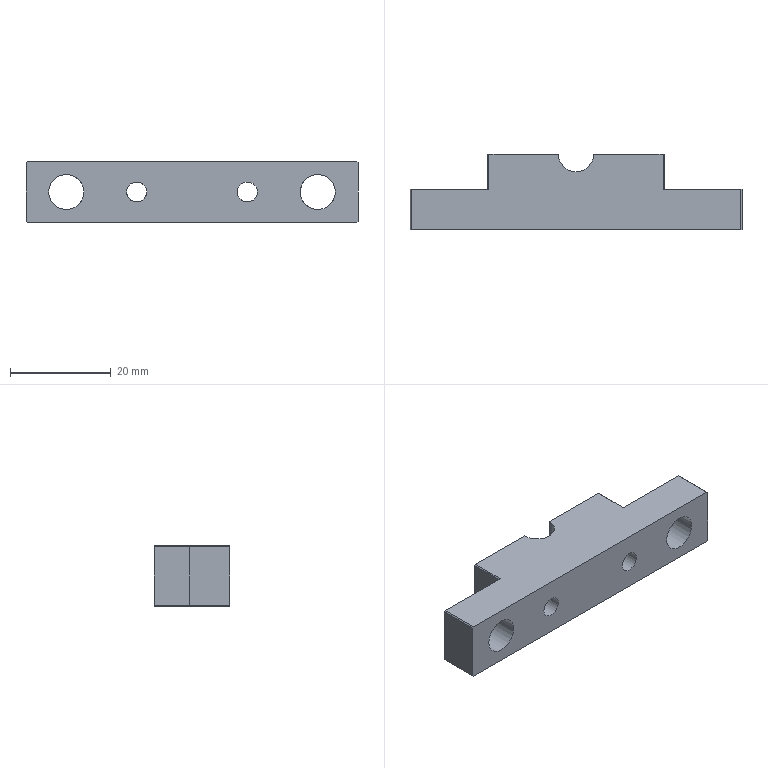NC program | NX | posted with a generic post | part box 66 x 15 x 12 mm
Whole program:
N10 G17 G21 G94 G90
(PLANAR_MILL , TOOL : D10开粗)
N12 T02 M6
N14 G54
N16 G17 G0 G90 X46.5 Y-3. B0. C0. S4500 M3
N18 G43 Z30. H2
N20 Z2.
N22 G94 G1 Z0. F1000.
N24 X36.5
N26 X-36.5
N28 X-46.5
N30 Z2.
N32 G0 Z30.
N34 X46.5 Y3.
N36 Z2.
N38 G1 Z0.
N40 X36.5
N42 X-36.5
N44 X-46.5
N46 Z2.
N48 G0 Z30.
(ADAPTIVE_MILLING , TOOL : D10开粗)
N50 X-32.154 Y-18.537 S5500
N52 Z-13.
N54 G1 X-32.171 Y-18.388 Z-13.937 F3000.
N56 X-32.188 Y-18.239 Z-14.308
N58 X-32.205 Y-18.09 Z-14.58
N60 X-32.222 Y-17.941 Z-14.8
N62 X-32.239 Y-17.791 Z-14.984
N64 X-32.255 Y-17.642 Z-15.142
N66 X-32.272 Y-17.493 Z-15.28
N68 X-32.289 Y-17.344 Z-15.4
N70 X-32.306 Y-17.195 Z-15.505
N72 X-32.323 Y-17.046 Z-15.598
N74 X-32.339 Y-16.897 Z-15.679
N76 X-32.356 Y-16.748 Z-15.75
N78 X-32.373 Y-16.599 Z-15.81
N80 X-32.39 Y-16.45 Z-15.862
N82 X-32.407 Y-16.301 Z-15.905
N84 X-32.424 Y-16.152 Z-15.939
N86 X-32.44 Y-16.003 Z-15.966
N88 X-32.457 Y-15.854 Z-15.985
N90 X-32.474 Y-15.705 Z-15.996
N92 X-32.491 Y-15.556 Z-16.
N94 X-32.687 Y-13.82
N96 G3 X-33.155 Y-13.077 R1.012
N98 X-34.636 Y-12.384 R5.494
N100 G2 X-37.759 Y-9.525 R6.545
N102 X-39.326 Y-4.936 R13.806
N104 X-39.908 Y3.097 R49.25
N106 X-39.899 Y5.158 R31.931
N108 X-37.912 Y8.459 R5.464
N110 G3 X-37.184 Y9.047 R22.941
N112 G2 X-34.827 Y10.897 R6.19
N114 X-32.799 Y11.3 R6.2
N116 X-22.302 Y11.491 R214.981
N118 G1 X-12.927 Y11.5
N120 X33.391 Y11.49
N122 G2 X36.639 Y9.788 R5.115
N124 X38.854 Y5.697 R9.985
N126 X39.767 Y-0.221 R27.104
N128 X39.889 Y-4.904 R50.965
N130 X38.038 Y-8.275 R5.243
N132 G1 X37.273 Y-8.915
N134 G2 X36.547 Y-9.748 R5.739
N136 X34.827 Y-10.897 R6.197
N138 X32.8 Y-11.3 R6.2
N140 X21.928 Y-11.492 R225.85
N142 G1 X12.928 Y-11.5
N144 X-29.01 Y-11.493
N146 G2 X-30.739 Y-11.3 R10.213
N148 X-33.493 Y-11.252 R28.791
N150 X-34.758 Y-10.925 R9.784
N152 G1 X-35.713 Y-10.428
N154 G2 X-37.407 Y-8.743 R7.579
N156 X-38.198 Y-6.833 R6.195
N158 G1 X-38.3 Y-5.799
N160 Y5.801
N162 G2 X-36.547 Y9.748 R5.488
N164 X-34.827 Y10.897 R6.197
N166 X-32.799 Y11.3 R6.2
N168 G1 X33.031 Y11.293
N170 X33.722 Y11.219
N172 X34.758 Y10.925
N174 X35.713 Y10.428
N176 G2 X37.335 Y8.849 R7.764
N178 X38.3 Y5.8 R5.571
N180 G1 Y-5.801
N182 G2 X36.547 Y-9.748 R5.489
N184 X34.827 Y-10.897 R6.197
N186 X32.8 Y-11.3 R6.2
N188 G1 X-30.763
N190 G3 X-31.772 Y-12.294 R1.01
N192 G1 X-31.796 Y-13.727
N194 X-31.798 Y-13.877 Z-15.996
N196 X-31.8 Y-14.027 Z-15.985
N198 X-31.803 Y-14.177 Z-15.966
N200 X-31.805 Y-14.326 Z-15.939
N202 X-31.808 Y-14.476 Z-15.905
N204 X-31.81 Y-14.626 Z-15.862
N206 X-31.813 Y-14.776 Z-15.81
N208 X-31.815 Y-14.926 Z-15.75
N210 X-31.818 Y-15.076 Z-15.679
N212 X-31.82 Y-15.226 Z-15.598
N214 X-31.822 Y-15.376 Z-15.505
N216 X-31.825 Y-15.526 Z-15.4
N218 X-31.827 Y-15.676 Z-15.28
N220 X-31.83 Y-15.826 Z-15.142
N222 X-31.832 Y-15.976 Z-14.984
N224 X-31.835 Y-16.126 Z-14.8
N226 X-31.837 Y-16.276 Z-14.58
N228 X-31.839 Y-16.426 Z-14.308
N230 X-31.842 Y-16.576 Z-13.937
N232 X-31.844 Y-16.726 Z-13.
N234 G0 Z30.
(PLANAR_MILL_1 , TOOL : D10开粗)
N236 X39.079 Y-11. S4500
N238 Z-14.
N240 G1 Z-16. F800.
N242 X32.799
N244 X-32.8
N246 G2 X-36.336 Y-9.536 R5.
N248 G1 X-36.536 Y-9.336
N250 G2 X-38. Y-5.8 R5.
N252 G1 Y5.8
N254 G2 X-36.536 Y9.336 R5.
N256 G1 X-36.336 Y9.536
N258 G2 X-32.8 Y11. R5.
N260 G1 X32.8
N262 G2 X36.336 Y9.536 R5.
N264 G1 X36.536 Y9.336
N266 G2 X38. Y5.8 R5.
N268 G1 Y-5.8
N270 G2 X36.536 Y-9.336 R5.
N272 G1 X36.336 Y-9.535
N274 X31.871 Y-14.
N276 Z-14.
N278 G0 Z30.
N280 X39.079 Y-11.
N282 Z-14.
N284 G1 Z-16.
N286 X32.799
N288 X-32.8
N290 G2 X-36.336 Y-9.536 R5.
N292 G1 X-36.536 Y-9.336
N294 G2 X-38. Y-5.8 R5.
N296 G1 Y5.8
N298 G2 X-36.536 Y9.336 R5.
N300 G1 X-36.336 Y9.536
N302 G2 X-32.8 Y11. R5.
N304 G1 X32.8
N306 G2 X36.336 Y9.536 R5.
N308 G1 X36.536 Y9.336
N310 G2 X38. Y5.8 R5.
N312 G1 Y-5.8
N314 G2 X36.536 Y-9.336 R5.
N316 G1 X36.336 Y-9.535
N318 X31.871 Y-14.
N320 Z-14.
N322 G0 Z30.
N324 X39.079 Y-11.
N326 Z-14.
N328 G1 Z-16.
N330 X32.799
N332 X-32.8
N334 G2 X-36.336 Y-9.536 R5.
N336 G1 X-36.536 Y-9.336
N338 G2 X-38. Y-5.8 R5.
N340 G1 Y5.8
N342 G2 X-36.536 Y9.336 R5.
N344 G1 X-36.336 Y9.536
N346 G2 X-32.8 Y11. R5.
N348 G1 X32.8
N350 G2 X36.336 Y9.536 R5.
N352 G1 X36.536 Y9.336
N354 G2 X38. Y5.8 R5.
N356 G1 Y-5.8
N358 G2 X36.536 Y-9.336 R5.
N360 G1 X36.336 Y-9.535
N362 X31.871 Y-14.
N364 Z-14.
N366 G0 Z30.
N368 M5
(PLANAR_MILL_1_COPY , TOOL : D8倒角刀)
N370 T04 M6
N372 G54
N374 G17 G0 G90 X36.341 Y-8. B0. C0. S4500 M3
N376 G43 Z30. H4
N378 Z0.
N380 G94 G1 Z-2. F800.
N382 X32.8
N384 X-32.8
N386 G2 X-34.214 Y-7.414 R2.
N388 G1 X-34.414 Y-7.214
N390 G2 X-35. Y-5.8 R2.
N392 G1 Y5.8
N394 G2 X-34.414 Y7.214 R2.
N396 G1 X-34.214 Y7.414
N398 G2 X-32.8 Y8. R2.
N400 G1 X32.8
N402 G2 X34.214 Y7.414 R2.
N404 G1 X34.414 Y7.214
N406 G2 X35. Y5.8 R2.
N408 G1 Y-5.8
N410 G2 X34.414 Y-7.214 R2.
N412 G1 X34.215 Y-7.414
N414 X31.628 Y-10.
N416 Z0.
N418 G0 Z30.
(DRILLING , TOOL : D8倒角刀)
N420 X-25. Y0. S3000
N422 G81 G98 Z-3.5 F200. R3.
N424 X25.
N426 G80
N428 G0 X25. Y0. Z30.
(DRILLING_COPY , TOOL : D8倒角刀)
N430 X-11.
N432 G81 Z-2.1 F200. R3.
N434 X11.
N436 G80
N438 G0 X11. Y0. Z30.
N440 M5
(PLANAR_MILL_COPY , TOOL : D63R0.8)
N442 T01 M6
N444 G54
N446 G17 G0 G90 X73. Y-3.5 B0. C0. S3500 M3
N448 G43 Z30. H1
N450 Z2.
N452 G94 G1 Z0. F600.
N454 X36.5
N456 X-36.5
N458 X-73.
N460 Z2.
N462 G0 Z30.
N464 M5
(DRILLING_COPY_1 , TOOL : D7钻头)
N466 T05 M6
N468 G54
N470 G17 G0 G90 X-25. Y0. B0. C0. S3000 M3
N472 G43 Z30. H5
N474 G94 G83 G98 Z-15. F200. Q2. R3.
N476 X25.
N478 G80
N480 G0 X25. Y0. Z30.
N482 M5
(HOLE_MILLING , TOOL : D4开粗)
N484 T08 M6
N486 G54
N488 G17 G0 G90 X-25. Y0. B0. C0. S4500 M3
N490 G43 Z30. H8
N492 Z-9.
N494 G94 G3 X-24.25 Y-0.75 R0.75 F200.
N496 X-23.5 Y0. R0.75
N498 X-25. Y1.5 R1.5
N500 X-23.5 Y0. R-1.5
N502 X-24.25 Y0.75 R0.75
N504 X-25. Y0. R0.75
N506 G0 Z30.
N508 X25.
N510 Z-9.
N512 G3 X25.75 Y-0.75 R0.75
N514 X26.5 Y0. R0.75
N516 X25. Y1.5 R1.5
N518 X26.5 Y0. R-1.5
N520 X25.75 Y0.75 R0.75
N522 X25. Y0. R0.75
N524 G0 Z30.
N526 M5
(DRILLING_COPY_COPY , TOOL : Z3.3)
N528 T06 M6
N530 G54
N532 G17 G0 G90 X-11. Y0. B0. C0. S3000 M3
N534 G43 Z30. H6
N536 G94 G83 G98 Z-18. F200. Q2. R3.
N538 X11.
N540 G80
N542 G0 X11. Y0. Z30.
N544 M5
(DRILLING_COPY_COPY_COPY , TOOL : M4X0.7)
N546 T07 M6
N548 G54
N550 G17 G0 G90 X-11. Y0. B0. C0. S300 M3
N552 G43 Z30. H7
N554 G84 G94 G98 Z-10. F210. R3.
N556 X11.
N558 G80
N560 G0 X11. Y0. Z30.
N562 M5
N564 M2